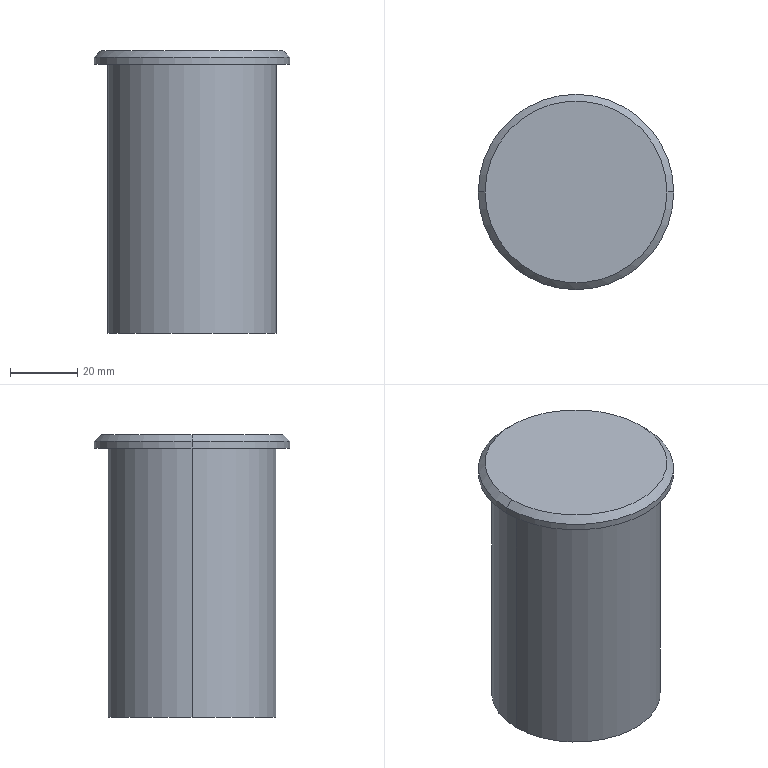Part | Creo | features DATUM PLANE 3, CURVE 2, PROTRUSION 2, CHAMFER 1, COORDINATE SYSTEM 1 | 1 solid | 9 faces | box 58 x 58 x 84 mm | volume 167292 mm3 | cylinder 4 | plane 3 | cone 2 | commonest cylinder face diameters 50 x2 58 x2
STEP:
#1=CARTESIAN_POINT('',(25.,0.,0.));
#2=VERTEX_POINT('',#1);
#3=CARTESIAN_POINT('',(-25.,0.,0.));
#4=VERTEX_POINT('',#3);
#5=CARTESIAN_POINT('',(0.,0.,0.));
#6=DIRECTION('',(0.,0.,1.));
#7=DIRECTION('',(1.,0.,0.));
#8=AXIS2_PLACEMENT_3D('',#5,#6,#7);
#9=CIRCLE('',#8,25.);
#10=EDGE_CURVE('',#2,#4,#9,.T.);
#11=ORIENTED_EDGE('',*,*,#10,.T.);
#12=CARTESIAN_POINT('',(0.,0.,0.));
#13=DIRECTION('',(0.,0.,1.));
#14=DIRECTION('',(-1.,0.,0.));
#15=AXIS2_PLACEMENT_3D('',#12,#13,#14);
#16=CIRCLE('',#15,25.);
#17=EDGE_CURVE('',#4,#2,#16,.T.);
#18=ORIENTED_EDGE('',*,*,#17,.T.);
#19=EDGE_LOOP('',(#11,#18));
#20=FACE_OUTER_BOUND('',#19,.F.);
#21=CARTESIAN_POINT('',(0.,0.,0.));
#22=DIRECTION('',(0.,0.,1.));
#23=DIRECTION('',(1.,0.,0.));
#24=AXIS2_PLACEMENT_3D('',#21,#22,#23);
#25=PLANE('',#24);
#26=ADVANCED_FACE('',(#20),#25,.F.);
#27=CARTESIAN_POINT('',(25.,0.,80.));
#28=VERTEX_POINT('',#27);
#29=CARTESIAN_POINT('',(-25.,0.,80.));
#30=VERTEX_POINT('',#29);
#31=CARTESIAN_POINT('',(0.,0.,80.));
#32=DIRECTION('',(0.,0.,1.));
#33=DIRECTION('',(1.,0.,0.));
#34=AXIS2_PLACEMENT_3D('',#31,#32,#33);
#35=CIRCLE('',#34,25.);
#36=EDGE_CURVE('',#28,#30,#35,.T.);
#37=ORIENTED_EDGE('',*,*,#36,.T.);
#38=CARTESIAN_POINT('',(-25.,0.,0.));
#39=DIRECTION('',(0.,0.,1.));
#40=VECTOR('',#39,80.);
#41=LINE('',#38,#40);
#42=EDGE_CURVE('',#4,#30,#41,.T.);
#43=ORIENTED_EDGE('',*,*,#42,.F.);
#44=ORIENTED_EDGE('',*,*,#10,.F.);
#45=CARTESIAN_POINT('',(25.,0.,0.));
#46=DIRECTION('',(0.,0.,1.));
#47=VECTOR('',#46,80.);
#48=LINE('',#45,#47);
#49=EDGE_CURVE('',#2,#28,#48,.T.);
#50=ORIENTED_EDGE('',*,*,#49,.T.);
#51=EDGE_LOOP('',(#37,#43,#44,#50));
#52=FACE_OUTER_BOUND('',#51,.F.);
#53=CARTESIAN_POINT('',(0.,0.,0.));
#54=DIRECTION('',(0.,0.,1.));
#55=DIRECTION('',(1.,0.,0.));
#56=AXIS2_PLACEMENT_3D('',#53,#54,#55);
#57=CYLINDRICAL_SURFACE('',#56,25.);
#58=ADVANCED_FACE('',(#52),#57,.T.);
#59=CARTESIAN_POINT('',(29.,0.,80.));
#60=VERTEX_POINT('',#59);
#61=CARTESIAN_POINT('',(-29.,0.,80.));
#62=VERTEX_POINT('',#61);
#63=CARTESIAN_POINT('',(0.,0.,80.));
#64=DIRECTION('',(0.,0.,1.));
#65=DIRECTION('',(1.,0.,0.));
#66=AXIS2_PLACEMENT_3D('',#63,#64,#65);
#67=CIRCLE('',#66,29.);
#68=EDGE_CURVE('',#60,#62,#67,.T.);
#69=ORIENTED_EDGE('',*,*,#68,.T.);
#70=CARTESIAN_POINT('',(0.,0.,80.));
#71=DIRECTION('',(0.,0.,1.));
#72=DIRECTION('',(-1.,0.,0.));
#73=AXIS2_PLACEMENT_3D('',#70,#71,#72);
#74=CIRCLE('',#73,29.);
#75=EDGE_CURVE('',#62,#60,#74,.T.);
#76=ORIENTED_EDGE('',*,*,#75,.T.);
#77=EDGE_LOOP('',(#69,#76));
#78=FACE_OUTER_BOUND('',#77,.F.);
#79=ORIENTED_EDGE('',*,*,#36,.F.);
#80=CARTESIAN_POINT('',(0.,0.,80.));
#81=DIRECTION('',(0.,0.,1.));
#82=DIRECTION('',(-1.,0.,0.));
#83=AXIS2_PLACEMENT_3D('',#80,#81,#82);
#84=CIRCLE('',#83,25.);
#85=EDGE_CURVE('',#30,#28,#84,.T.);
#86=ORIENTED_EDGE('',*,*,#85,.F.);
#87=EDGE_LOOP('',(#79,#86));
#88=FACE_BOUND('',#87,.F.);
#89=CARTESIAN_POINT('',(0.,0.,80.));
#90=DIRECTION('',(0.,0.,1.));
#91=DIRECTION('',(1.,0.,0.));
#92=AXIS2_PLACEMENT_3D('',#89,#90,#91);
#93=PLANE('',#92);
#94=ADVANCED_FACE('',(#78,#88),#93,.F.);
#95=CARTESIAN_POINT('',(29.,0.,82.));
#96=VERTEX_POINT('',#95);
#97=CARTESIAN_POINT('',(-29.,0.,82.));
#98=VERTEX_POINT('',#97);
#99=CARTESIAN_POINT('',(0.,0.,82.));
#100=DIRECTION('',(0.,0.,1.));
#101=DIRECTION('',(1.,0.,0.));
#102=AXIS2_PLACEMENT_3D('',#99,#100,#101);
#103=CIRCLE('',#102,29.);
#104=EDGE_CURVE('',#96,#98,#103,.T.);
#105=ORIENTED_EDGE('',*,*,#104,.T.);
#106=CARTESIAN_POINT('',(-29.,0.,80.));
#107=DIRECTION('',(0.,-0.000000002,1.));
#108=VECTOR('',#107,2.);
#109=LINE('',#106,#108);
#110=EDGE_CURVE('',#62,#98,#109,.T.);
#111=ORIENTED_EDGE('',*,*,#110,.F.);
#112=ORIENTED_EDGE('',*,*,#68,.F.);
#113=CARTESIAN_POINT('',(29.,0.,80.));
#114=DIRECTION('',(0.,0.000000002,1.));
#115=VECTOR('',#114,2.);
#116=LINE('',#113,#115);
#117=EDGE_CURVE('',#60,#96,#116,.T.);
#118=ORIENTED_EDGE('',*,*,#117,.T.);
#119=EDGE_LOOP('',(#105,#111,#112,#118));
#120=FACE_OUTER_BOUND('',#119,.F.);
#121=CARTESIAN_POINT('',(0.,0.,80.));
#122=DIRECTION('',(0.,0.,1.));
#123=DIRECTION('',(1.,0.,0.));
#124=AXIS2_PLACEMENT_3D('',#121,#122,#123);
#125=CYLINDRICAL_SURFACE('',#124,29.);
#126=ADVANCED_FACE('',(#120),#125,.T.);
#127=CARTESIAN_POINT('',(27.,0.,84.));
#128=VERTEX_POINT('',#127);
#129=CARTESIAN_POINT('',(-27.,0.,84.));
#130=VERTEX_POINT('',#129);
#131=CARTESIAN_POINT('',(0.,0.,84.));
#132=DIRECTION('',(0.,0.,1.));
#133=DIRECTION('',(1.,0.,0.));
#134=AXIS2_PLACEMENT_3D('',#131,#132,#133);
#135=CIRCLE('',#134,27.);
#136=EDGE_CURVE('',#128,#130,#135,.T.);
#137=ORIENTED_EDGE('',*,*,#136,.T.);
#138=CARTESIAN_POINT('',(-27.,-0.000000006,84.));
#139=DIRECTION('',(-0.7071,0.,-0.7071));
#140=VECTOR('',#139,2.828);
#141=LINE('',#138,#140);
#142=EDGE_CURVE('',#130,#98,#141,.T.);
#143=ORIENTED_EDGE('',*,*,#142,.T.);
#144=ORIENTED_EDGE('',*,*,#104,.F.);
#145=CARTESIAN_POINT('',(27.,0.000000006,84.));
#146=DIRECTION('',(0.7071,0.,-0.7071));
#147=VECTOR('',#146,2.828);
#148=LINE('',#145,#147);
#149=EDGE_CURVE('',#128,#96,#148,.T.);
#150=ORIENTED_EDGE('',*,*,#149,.F.);
#151=EDGE_LOOP('',(#137,#143,#144,#150));
#152=FACE_OUTER_BOUND('',#151,.F.);
#153=CARTESIAN_POINT('',(0.,0.,83.));
#154=DIRECTION('',(0.,0.,-1.));
#155=DIRECTION('',(0.,-1.,0.));
#156=AXIS2_PLACEMENT_3D('',#153,#154,#155);
#157=CONICAL_SURFACE('',#156,28.,45.);
#158=ADVANCED_FACE('',(#152),#157,.T.);
#159=CARTESIAN_POINT('',(0.,0.,84.));
#160=DIRECTION('',(0.,0.,1.));
#161=DIRECTION('',(-1.,0.,0.));
#162=AXIS2_PLACEMENT_3D('',#159,#160,#161);
#163=CIRCLE('',#162,27.);
#164=EDGE_CURVE('',#130,#128,#163,.T.);
#165=ORIENTED_EDGE('',*,*,#164,.F.);
#166=ORIENTED_EDGE('',*,*,#136,.F.);
#167=EDGE_LOOP('',(#165,#166));
#168=FACE_OUTER_BOUND('',#167,.F.);
#169=CARTESIAN_POINT('',(0.,0.,84.));
#170=DIRECTION('',(0.,0.,1.));
#171=DIRECTION('',(1.,0.,0.));
#172=AXIS2_PLACEMENT_3D('',#169,#170,#171);
#173=PLANE('',#172);
#174=ADVANCED_FACE('',(#168),#173,.T.);
#175=ORIENTED_EDGE('',*,*,#164,.T.);
#176=ORIENTED_EDGE('',*,*,#149,.T.);
#177=CARTESIAN_POINT('',(0.,0.,82.));
#178=DIRECTION('',(0.,0.,1.));
#179=DIRECTION('',(-1.,0.,0.));
#180=AXIS2_PLACEMENT_3D('',#177,#178,#179);
#181=CIRCLE('',#180,29.);
#182=EDGE_CURVE('',#98,#96,#181,.T.);
#183=ORIENTED_EDGE('',*,*,#182,.F.);
#184=ORIENTED_EDGE('',*,*,#142,.F.);
#185=EDGE_LOOP('',(#175,#176,#183,#184));
#186=FACE_OUTER_BOUND('',#185,.F.);
#187=CARTESIAN_POINT('',(0.,0.,83.));
#188=DIRECTION('',(0.,0.,-1.));
#189=DIRECTION('',(0.,-1.,0.));
#190=AXIS2_PLACEMENT_3D('',#187,#188,#189);
#191=CONICAL_SURFACE('',#190,28.,45.);
#192=ADVANCED_FACE('',(#186),#191,.T.);
#193=ORIENTED_EDGE('',*,*,#182,.T.);
#194=ORIENTED_EDGE('',*,*,#117,.F.);
#195=ORIENTED_EDGE('',*,*,#75,.F.);
#196=ORIENTED_EDGE('',*,*,#110,.T.);
#197=EDGE_LOOP('',(#193,#194,#195,#196));
#198=FACE_OUTER_BOUND('',#197,.F.);
#199=CARTESIAN_POINT('',(0.,0.,80.));
#200=DIRECTION('',(0.,0.,1.));
#201=DIRECTION('',(1.,0.,0.));
#202=AXIS2_PLACEMENT_3D('',#199,#200,#201);
#203=CYLINDRICAL_SURFACE('',#202,29.);
#204=ADVANCED_FACE('',(#198),#203,.T.);
#205=ORIENTED_EDGE('',*,*,#85,.T.);
#206=ORIENTED_EDGE('',*,*,#49,.F.);
#207=ORIENTED_EDGE('',*,*,#17,.F.);
#208=ORIENTED_EDGE('',*,*,#42,.T.);
#209=EDGE_LOOP('',(#205,#206,#207,#208));
#210=FACE_OUTER_BOUND('',#209,.F.);
#211=CARTESIAN_POINT('',(0.,0.,0.));
#212=DIRECTION('',(0.,0.,1.));
#213=DIRECTION('',(1.,0.,0.));
#214=AXIS2_PLACEMENT_3D('',#211,#212,#213);
#215=CYLINDRICAL_SURFACE('',#214,25.);
#216=ADVANCED_FACE('',(#210),#215,.T.);
#217=CLOSED_SHELL('',(#26,#58,#94,#126,#158,#174,#192,#204,#216));
#218=MANIFOLD_SOLID_BREP('',#217);
#219=(LENGTH_UNIT()NAMED_UNIT(*)SI_UNIT(.MILLI.,.METRE.));
#220=UNCERTAINTY_MEASURE_WITH_UNIT(LENGTH_MEASURE(0.01174),#219,'','');
#221=(NAMED_UNIT(*)PLANE_ANGLE_UNIT()SI_UNIT($,.RADIAN.));
#222=PLANE_ANGLE_MEASURE_WITH_UNIT(PLANE_ANGLE_MEASURE(0.01745),#221);
#223=(CONVERSION_BASED_UNIT('DEGREE',#222)NAMED_UNIT(*)PLANE_ANGLE_UNIT());
#224=(NAMED_UNIT(*)SI_UNIT($,.STERADIAN.)SOLID_ANGLE_UNIT());
#225=(GEOMETRIC_REPRESENTATION_CONTEXT(3)GLOBAL_UNCERTAINTY_ASSIGNED_CONTEXT((#220))GLOBAL_UNIT_ASSIGNED_CONTEXT((#219,#223,#224))REPRESENTATION_CONTEXT('',''));
#226=ADVANCED_BREP_SHAPE_REPRESENTATION('',(#218),#225);